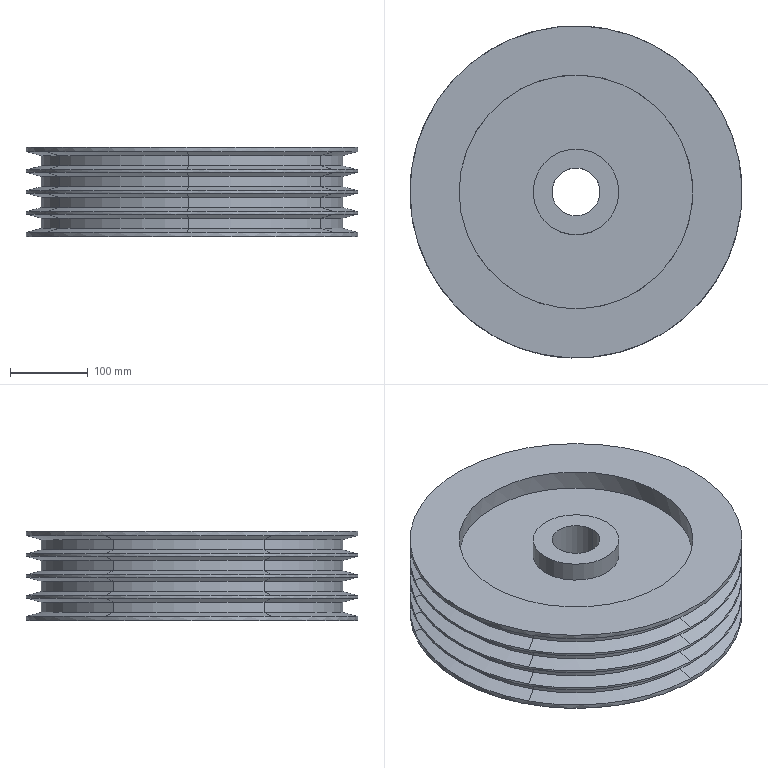Part | NX | features DATUM_CSYS 1, LINKED_BODY 1 | 1 solid | 89 faces | box 426.001 x 426 x 114.878 mm | volume 11128143 mm3 | spline 72 | cylinder 11 | plane 6 | commonest cylinder face diameters 426 x5 61.44 x2 110 x2 300 x2